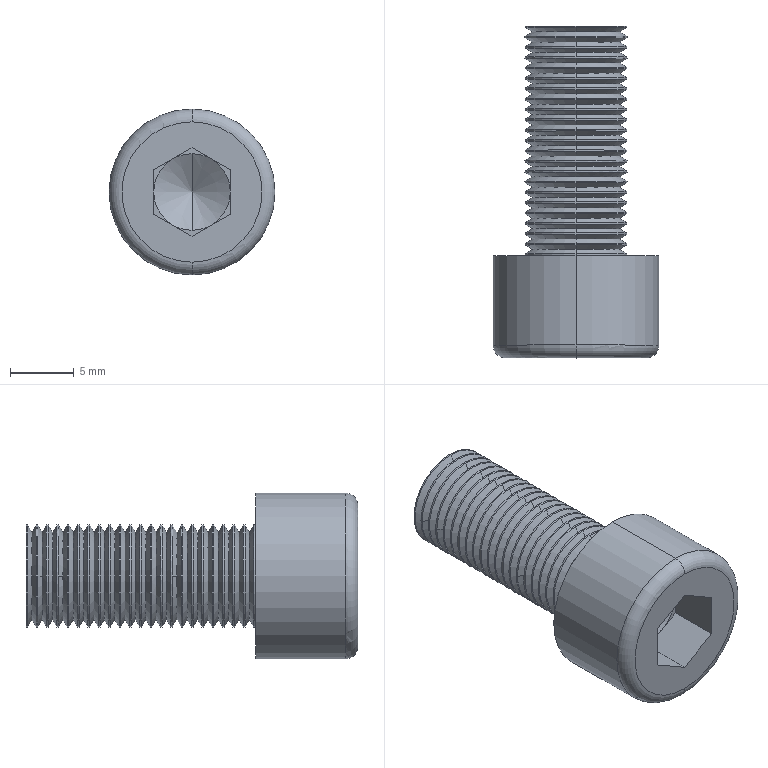Part | SolidWorks | features BaseBody 1 | 1 solid | 155 faces | box 13 x 26 x 13 mm | volume 1713 mm3 | cone 90 | cylinder 48 | plane 15 | torus 2 | commonest cylinder face diameters 8 x46 13 x2